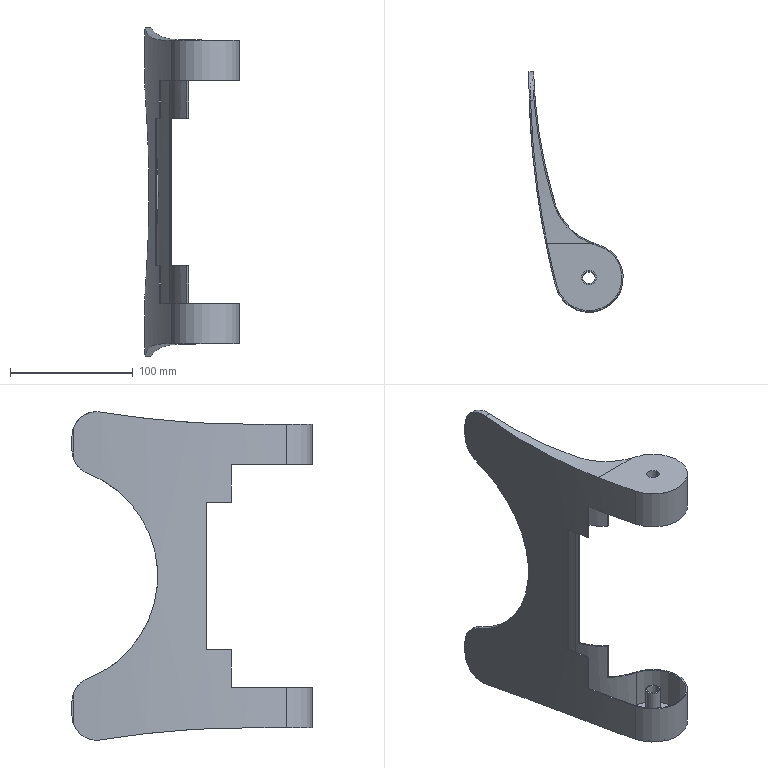Part | SolidWorks | features ICE 3, Extrusion 1, Shell 1 | 1 solid | 60 faces | box 77.001 x 196 x 268.141 mm | volume 67561 mm3 | cylinder 38 | plane 22 | commonest cylinder face diameters 38 x5 40 x5 1400 x5 10 x4 12 x4 1398 x3